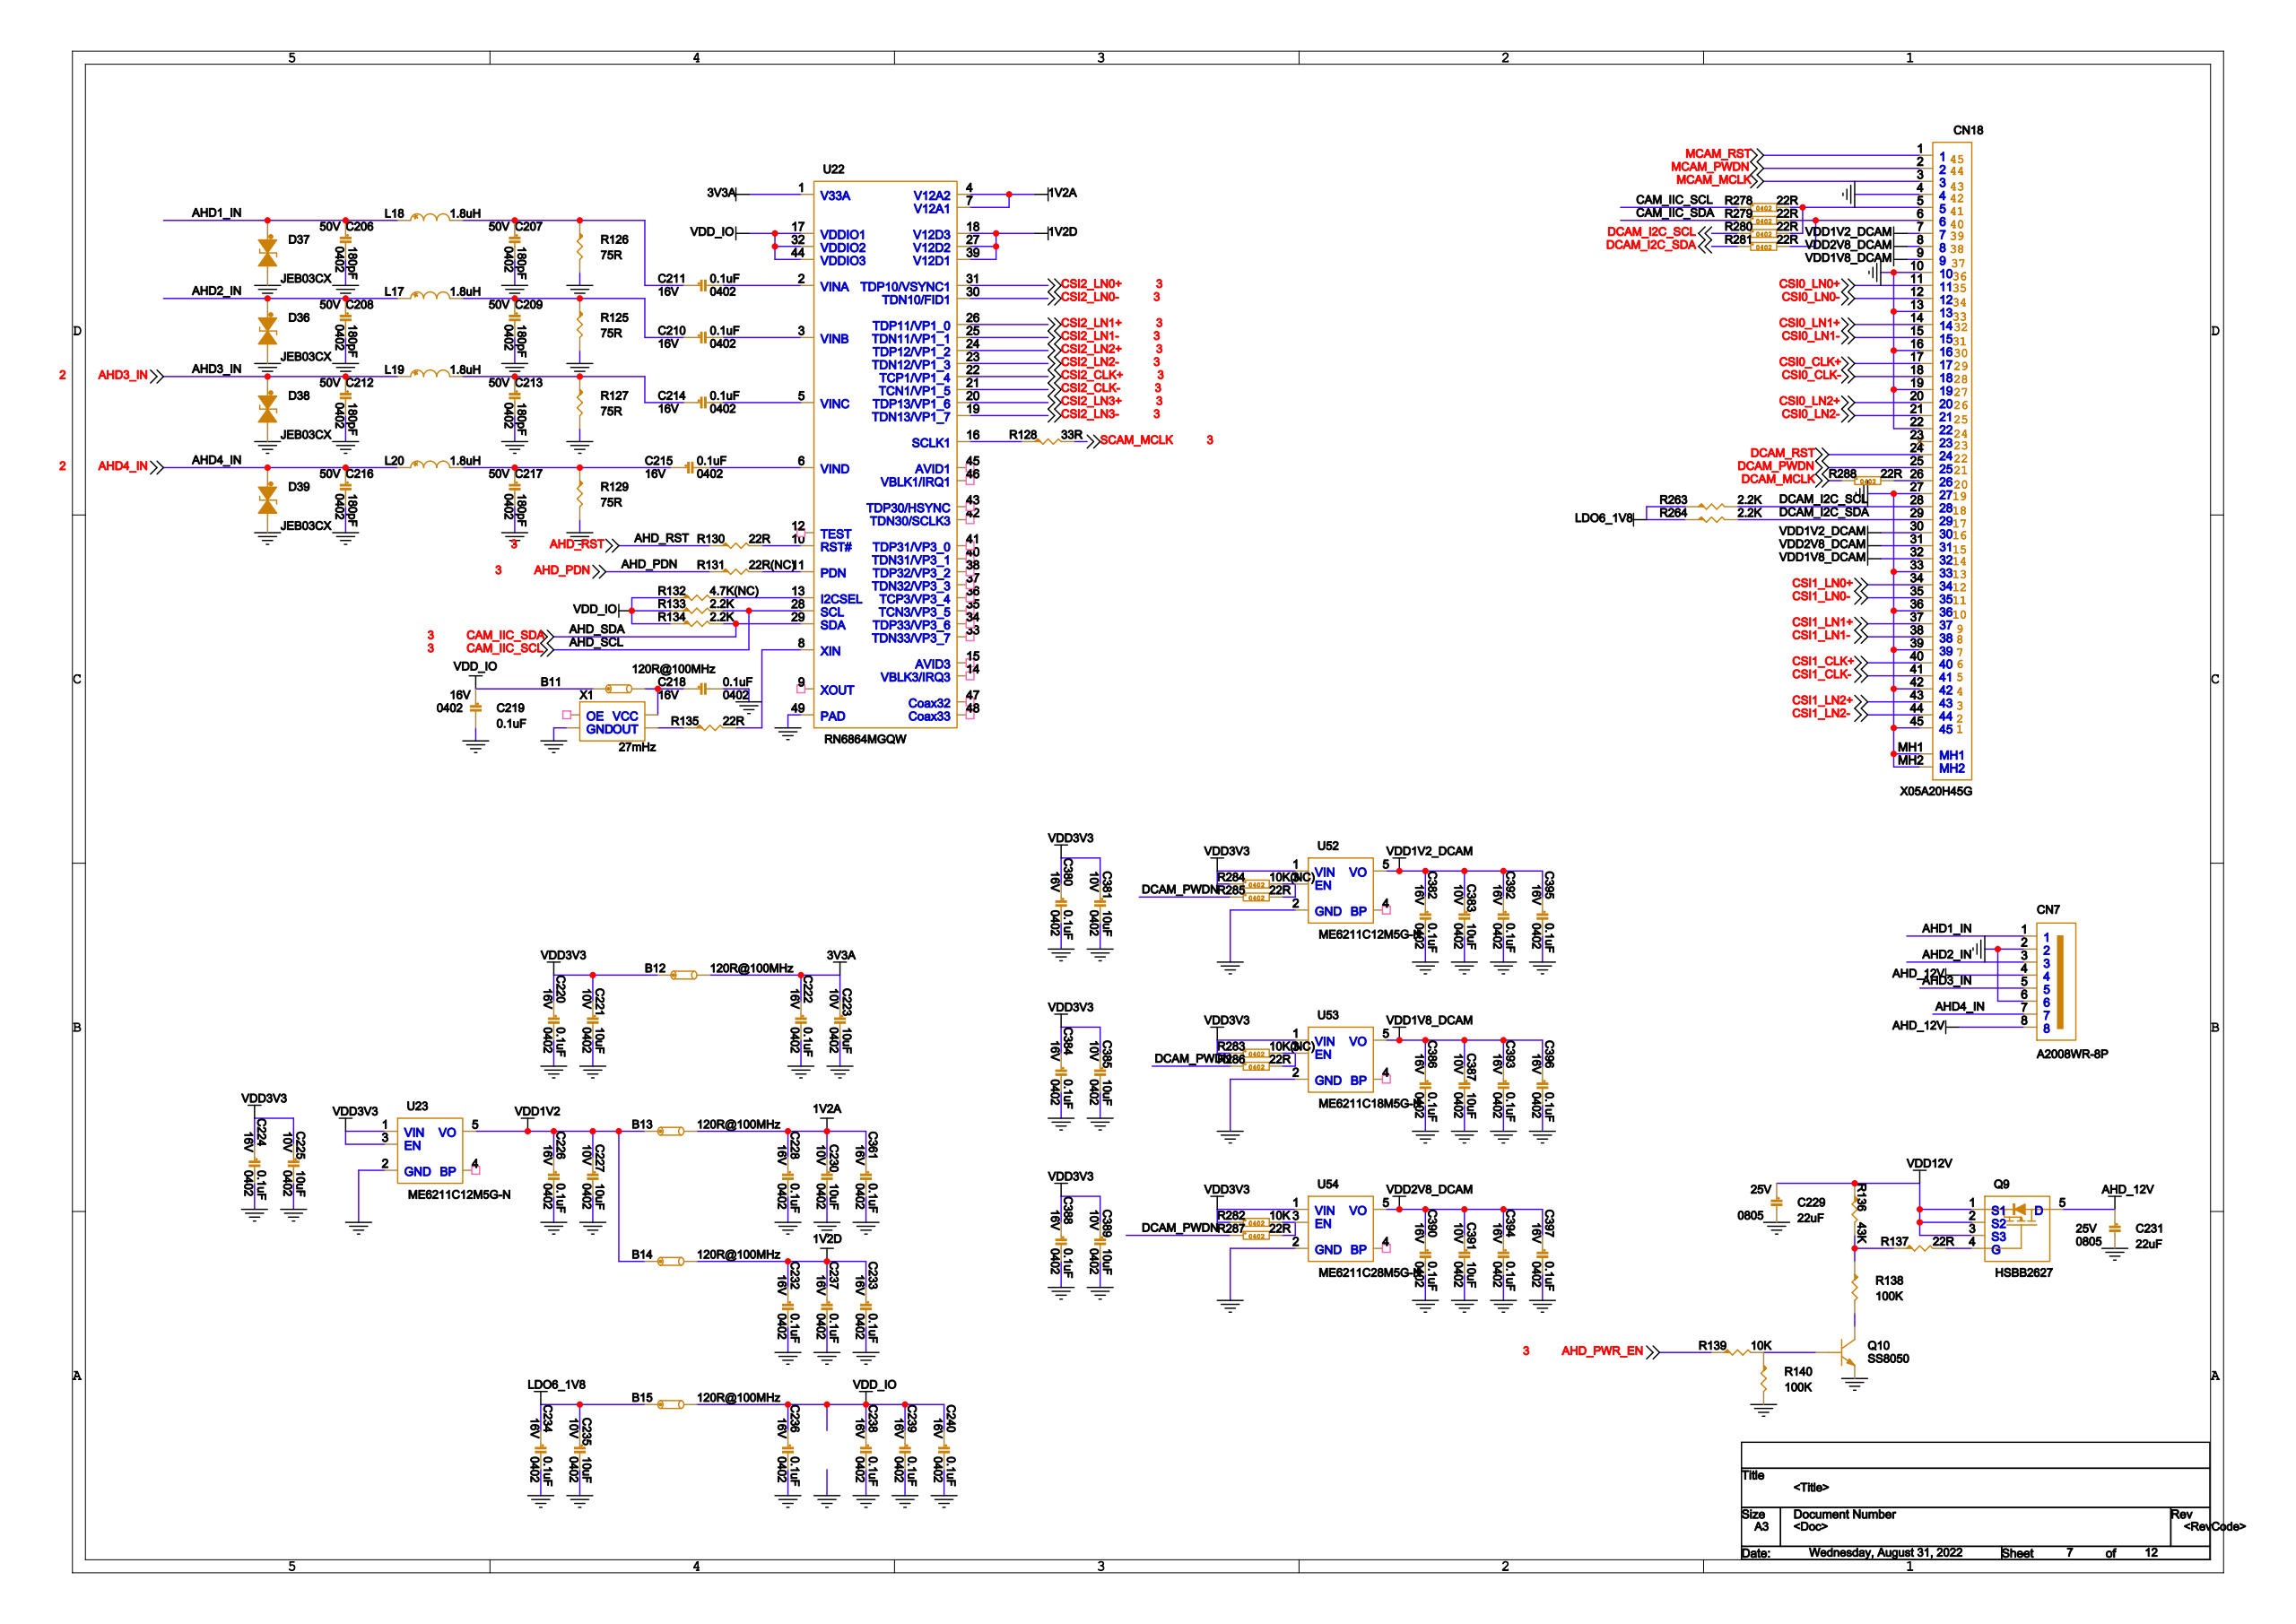Circuit board | Cadence Allegro | 970 parts | 627 nets | one sheet of the schematic
Parts on this sheet (reference | value | footprint):
B11 | 120R@100MHz | R0402
B12 | 120R@100MHz | R0402
B13 | 120R@100MHz | R0402
B14 | 120R@100MHz | R0402
B15 | 120R@100MHz | R0402
C206 | 180pF | C0402
C207 | 180pF | C0402
C208 | 180pF | C0402
C209 | 180pF | C0402
C210 | 0.1uF | C0402
C211 | 0.1uF | C0402
C212 | 180pF | C0402
C213 | 180pF | C0402
C214 | 0.1uF | C0402
C215 | 0.1uF | C0402
C216 | 180pF | C0402
C217 | 180pF | C0402
C218 | 0.1uF | C0402
C219 | 0.1uF | C0402
C220 | 0.1uF | C0402
C221 | 10uF | C0402
C222 | 0.1uF | C0402
C223 | 10uF | C0402
C224 | 0.1uF | C0402
C225 | 10uF | C0402
C226 | 0.1uF | C0402
C227 | 10uF | C0402
C228 | 0.1uF | C0402
C229 | 22uF | C0805
C230 | 10uF | C0402
C231 | 22uF | C0805
C232 | 0.1uF | C0402
C233 | 0.1uF | C0402
C234 | 0.1uF | C0402
C235 | 10uF | C0402
C236 | 0.1uF | C0402
C237 | 0.1uF | C0402
C238 | 0.1uF | C0402
C239 | 0.1uF | C0402
C240 | 0.1uF | C0402
C361 | 0.1uF | C0402
C380 | 0.1uF | C0402
C381 | 10uF | C0402
C382 | 0.1uF | C0402
C383 | 10uF | C0402
C384 | 0.1uF | C0402
C385 | 10uF | C0402
C386 | 0.1uF | C0402
C387 | 10uF | C0402
C388 | 0.1uF | C0402
C389 | 10uF | C0402
C390 | 0.1uF | C0402
C391 | 10uF | C0402
C392 | 0.1uF | C0402
C393 | 0.1uF | C0402
C394 | 0.1uF | C0402
C395 | 0.1uF | C0402
C396 | 0.1uF | C0402
C397 | 0.1uF | C0402
CN7 | A2008WR-8P | A2008WR_8P
CN18 | X05A20H45G | FPC-45-0P5-2MMH
D36 | JEB03CX | SOD-323
D37 | JEB03CX | SOD-323
D38 | JEB03CX | SOD-323
D39 | JEB03CX | SOD-323
L17 | 1.8uH | R0603
L18 | 1.8uH | R0603
L19 | 1.8uH | R0603
L20 | 1.8uH | R0603
Q9 | HSBB2627 | DFN3X3
Q10 | SS8050 | SOT-23
R125 | 75R | R0402
R126 | 75R | R0402
R127 | 75R | R0402
R128 | 33R | R0402
R129 | 75R | R0402
R130 | 22R | R0402
R131 | 22R(NC) | R0402
R132 | 4.7K(NC) | R0402
R133 | 2.2K | R0402
R134 | 2.2K | R0402
R135 | 22R | R0402
R136 | 43K | R0402
R137 | 22R | R0402
R138 | 100K | R0402
R139 | 10K | R0402
R140 | 100K | R0402
R263 | 2.2K | R0402
R264 | 2.2K | R0402
R278 | 22R | R0402
R279 | 22R | R0402
R280 | 22R | R0402
R281 | 22R | R0402
R282 | 10K | R0402
R283 | 10K | R0402
R284 | 10K | R0402
R285 | 22R | R0402
R286 | 22R | R0402
R287 | 22R | R0402
R288 | 22R | R0402
U22 | RN6864MGQW | QFN48_0P4_6X6MM_EPAD
U23 | ME6211C12M5G-N | SOT23-5
U52 | ME6211C12M5G-N | SOT23-5
U53 | ME6211C18M5G-N | SOT23-5
U54 | ME6211C28M5G-N | SOT23-5
X1 | 27mHz | X3225
Nets of these parts (net: part-pin ...):
VDD3V3: B12-1 C220-1 C221-1 C224-1 C225-1 C380-1 C381-1 C384-1 C385-1 C388-1 C389-1 R282-1 R283-1 R284-1 U23-1 U23-3 U52-1 U53-1 U54-1
GND: C206-2 C207-2 C208-2 C209-2 C212-2 C213-2 C216-2 C217-2 C218-2 C219-2 C220-2 C221-2 C222-2 C223-2 C224-2 C225-2 C226-2 C227-2 C228-2 C229-2 C230-2 C231-2 C232-2 C233-2 C234-2 C235-2 C236-2 C237-2 C238-2 C239-2 C240-2 C361-2 C380-2 C381-2 C382-2 C383-2 C384-2 C385-2 C386-2 C387-2 C388-2 C389-2 C390-2 C391-2 C392-2 C393-2 C394-2 C395-2 C396-2 C397-2 CN7-2 CN7-6 D36-1 D37-1 D38-1 D39-1 Q10-2 R125-2 R126-2 R127-2 R129-2 R140-2 U23-2 U52-2 U53-2 U54-2 X1-2 CN18-4 CN18-10 CN18-13 CN18-16 CN18-19 CN18-22 CN18-27 CN18-33 CN18-36 CN18-39 CN18-42 CN18-45 CN18-MH1 CN18-MH2 U22-49
LDO6_1V8: B15-1 C234-1 C235-1 R263-1 R264-1
AHD1_IN: C206-1 CN7-1 D37-2 L18-1
AHD2_IN: C208-1 CN7-3 D36-2 L17-1
AHD_12V: C231-1 CN7-4 CN7-8 Q9-5
AHD3_IN: C212-1 CN7-5 D38-2 L19-1
AHD4_IN: C216-1 CN7-7 D39-2 L20-1
N19686614: R282-2 R287-2 U54-3
N19686540: R283-2 R286-2 U53-3
N19686471: R284-2 R285-2 U52-3
VDD1V8_DCAM: C386-1 C387-1 C393-1 C396-1 U53-5 CN18-9 CN18-32
VDD2V8_DCAM: C390-1 C391-1 C394-1 C397-1 U54-5 CN18-8 CN18-31
MCAM_RST: CN18-1
CSI0_LN0-: CN18-12
CSI0_LN1+: CN18-14
CSI0_LN1-: CN18-15
CSI0_CLK+: CN18-17
MCAM_PWDN: CN18-2
CSI0_LN2+: CN18-20
CSI0_LN2-: CN18-21
DCAM_RST: CN18-24
DCAM_PWDN: R285-1 R286-1 R287-1 CN18-25
N19690134: R288-2 CN18-26
DCAM_I2C_SCL: R263-2 R280-1 CN18-28
DCAM_I2C_SDA: R264-2 R281-1 CN18-29
MCAM_MCLK: CN18-3
VDD1V2_DCAM: C382-1 C383-1 C392-1 C395-1 U52-5 CN18-7 CN18-30
CSI1_LN0-: CN18-35
CSI1_LN1+: CN18-37
CSI1_LN1-: CN18-38
CSI1_CLK+: CN18-40
CSI1_LN2+: CN18-43
CSI1_LN2-: CN18-44
N19681313: R278-2 R280-2 CN18-5
N19681316: R279-2 R281-2 CN18-6
VDD12V: C229-1 Q9-1 Q9-2 Q9-3 R136-1
CAM_IIC_SCL: R133-2 R278-1 U22-28
CAM_IIC_SDA: R134-2 R279-1 U22-29
DCAM_MCLK: R288-1
AHD_PDN: R131-1
N19285933: R131-2 U22-11
N19286330: R135-1 X1-3
N19286439: B11-2 C218-1 X1-4
N19286062: R132-2 U22-13
N19285850: R130-2 U22-10
N19296265: R128-1 U22-16
CSI2_CLK-: U22-21
CSI2_CLK+: U22-22
CSI2_LN0-: U22-30
CSI2_LN1-: U22-25
CSI2_LN2-: U22-23
CSI2_LN3-: U22-19
CSI2_LN0+: U22-31
CSI2_LN1+: U22-26
CSI2_LN2+: U22-24
CSI2_LN3+: U22-20
1V2A: B13-2 C228-1 C230-1 C361-1 U22-4 U22-7
1V2D: B14-2 C232-1 C233-1 C237-1 U22-18 U22-27 U22-39
3V3A: B12-2 C222-1 C223-1 U22-1
VDD_IO: B11-1 B15-2 C219-1 C236-1 C238-1 C239-1 C240-1 R132-1 R133-1 R134-1 U22-17 U22-32 U22-44
N19285010: C211-2 U22-2
N19285313: C210-2 U22-3
N19285552: C214-2 U22-5
N19285732: C215-2 U22-6
N19286333: R135-2 U22-8
VDD1V2: B13-1 B14-1 C226-1 C227-1 U23-5
N19285026: C207-1 C211-1 L18-2 R126-1
N19285315: C209-1 C210-1 L17-2 R125-1
N19285554: C213-1 C214-1 L19-2 R127-1
N19285734: C215-1 C217-1 L20-2 R129-1
N19305985: Q10-1 R139-2 R140-1
N19306230: Q10-3 R138-2
N19306130: Q9-4 R137-2
N19305905: R136-2 R137-1 R138-1
AHD_RST: R130-1
AHD_PWR_EN: R139-1
SCAM_MCLK: R128-2